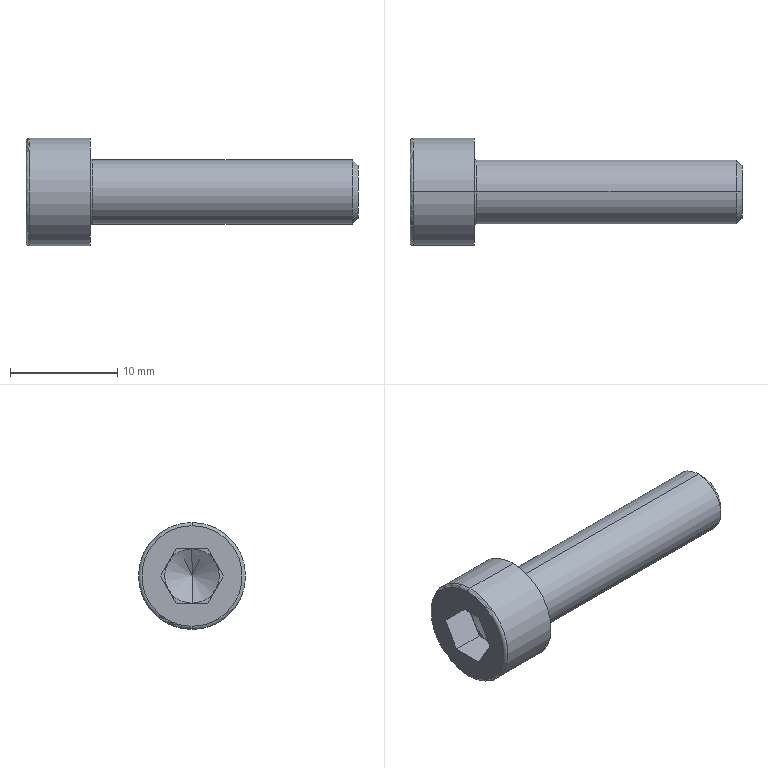Part | STEP file | socket head cap screw_iso_ISO 4762 M6 x 25 --- 25N | 1 solid | 27 faces | box 31 x 10 x 10 mm | volume 1098 mm3 | plane 15 | cone 4 | torus 4 | cylinder 4 | commonest cylinder face diameters 6 x2 10 x2